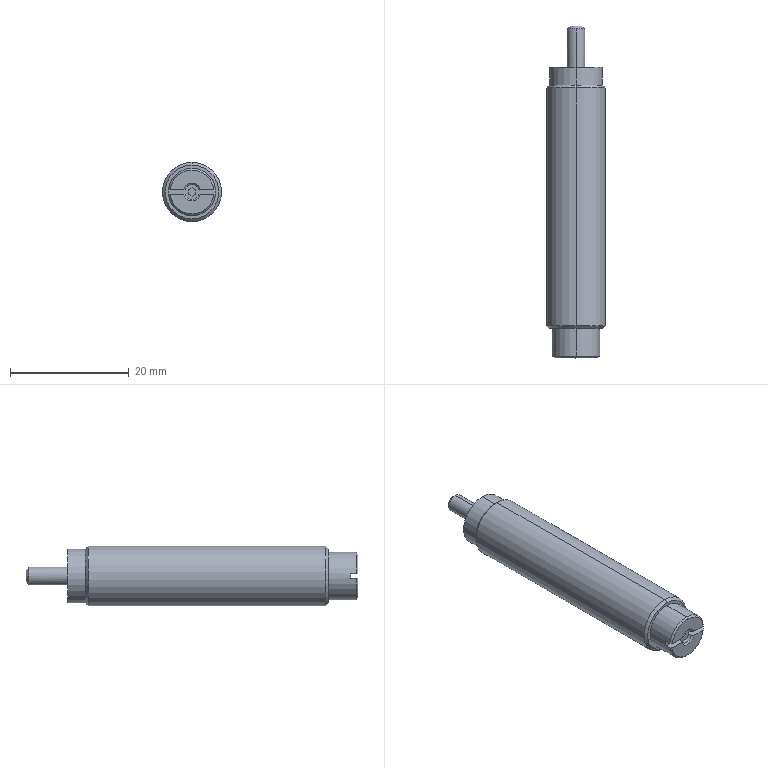Part | STEP file | 11-_ACA-1007-2-N_Body11 | 1 solid | 41 faces | box 10 x 56 x 10 mm | volume 3690 mm3 | plane 18 | cone 13 | cylinder 10 | commonest cylinder face diameters 2.459 x2 3 x2 8 x2 9 x2 10 x2
STEP:
#1=CARTESIAN_POINT('',(0.,5.46,5.));
#2=VERTEX_POINT('',#1);
#3=CARTESIAN_POINT('',(0.,5.46,-5.));
#4=VERTEX_POINT('',#3);
#5=CARTESIAN_POINT('',(0.,5.46,0.));
#6=DIRECTION('',(0.,1.,0.));
#7=DIRECTION('',(0.,0.,1.));
#8=AXIS2_PLACEMENT_3D('',#5,#6,#7);
#9=CIRCLE('',#8,5.);
#10=EDGE_CURVE('',#2,#4,#9,.T.);
#11=ORIENTED_EDGE('',*,*,#10,.T.);
#12=CARTESIAN_POINT('',(0.,45.54,-5.));
#13=VERTEX_POINT('',#12);
#14=CARTESIAN_POINT('',(0.,0.,-5.));
#15=DIRECTION('',(0.,1.,0.));
#16=VECTOR('',#15,1000.);
#17=LINE('',#14,#16);
#18=EDGE_CURVE('',#4,#13,#17,.T.);
#19=ORIENTED_EDGE('',*,*,#18,.T.);
#20=CARTESIAN_POINT('',(0.,45.54,5.));
#21=VERTEX_POINT('',#20);
#22=CARTESIAN_POINT('',(0.,45.54,0.));
#23=DIRECTION('',(0.,-1.,0.));
#24=DIRECTION('',(0.,0.,1.));
#25=AXIS2_PLACEMENT_3D('',#22,#23,#24);
#26=CIRCLE('',#25,5.);
#27=EDGE_CURVE('',#13,#21,#26,.T.);
#28=ORIENTED_EDGE('',*,*,#27,.T.);
#29=CARTESIAN_POINT('',(0.,0.,5.));
#30=DIRECTION('',(0.,1.,0.));
#31=VECTOR('',#30,1000.);
#32=LINE('',#29,#31);
#33=EDGE_CURVE('',#2,#21,#32,.T.);
#34=ORIENTED_EDGE('',*,*,#33,.F.);
#35=EDGE_LOOP('',(#11,#19,#28,#34));
#36=FACE_OUTER_BOUND('',#35,.T.);
#37=CARTESIAN_POINT('',(0.,0.,0.));
#38=DIRECTION('',(0.,1.,0.));
#39=DIRECTION('',(0.,0.,1.));
#40=AXIS2_PLACEMENT_3D('',#37,#38,#39);
#41=CYLINDRICAL_SURFACE('',#40,5.);
#42=ADVANCED_FACE('',(#36),#41,.T.);
#43=CARTESIAN_POINT('',(0.,46.,-4.54));
#44=VERTEX_POINT('',#43);
#45=CARTESIAN_POINT('',(0.,46.,4.54));
#46=VERTEX_POINT('',#45);
#47=CARTESIAN_POINT('',(0.,46.,0.));
#48=DIRECTION('',(0.,-1.,0.));
#49=DIRECTION('',(0.,0.,-1.));
#50=AXIS2_PLACEMENT_3D('',#47,#48,#49);
#51=CIRCLE('',#50,4.54);
#52=EDGE_CURVE('',#44,#46,#51,.T.);
#53=ORIENTED_EDGE('',*,*,#52,.T.);
#54=CARTESIAN_POINT('',(0.,45.54,5.));
#55=DIRECTION('',(0.,-0.7071,0.7071));
#56=VECTOR('',#55,1000.);
#57=LINE('',#54,#56);
#58=EDGE_CURVE('',#46,#21,#57,.T.);
#59=ORIENTED_EDGE('',*,*,#58,.T.);
#60=ORIENTED_EDGE('',*,*,#27,.F.);
#61=CARTESIAN_POINT('',(0.,45.54,-5.));
#62=DIRECTION('',(0.,-0.7071,-0.7071));
#63=VECTOR('',#62,1000.);
#64=LINE('',#61,#63);
#65=EDGE_CURVE('',#44,#13,#64,.T.);
#66=ORIENTED_EDGE('',*,*,#65,.F.);
#67=EDGE_LOOP('',(#53,#59,#60,#66));
#68=FACE_OUTER_BOUND('',#67,.T.);
#69=CARTESIAN_POINT('',(0.,45.54,0.));
#70=DIRECTION('',(0.,-1.,0.));
#71=DIRECTION('',(0.,0.,-1.));
#72=AXIS2_PLACEMENT_3D('',#69,#70,#71);
#73=CONICAL_SURFACE('',#72,5.,0.7854);
#74=ADVANCED_FACE('',(#68),#73,.T.);
#75=CARTESIAN_POINT('',(0.,5.,4.54));
#76=VERTEX_POINT('',#75);
#77=CARTESIAN_POINT('',(0.,5.,-4.54));
#78=VERTEX_POINT('',#77);
#79=CARTESIAN_POINT('',(0.,5.,0.));
#80=DIRECTION('',(0.,1.,0.));
#81=DIRECTION('',(0.,0.,1.));
#82=AXIS2_PLACEMENT_3D('',#79,#80,#81);
#83=CIRCLE('',#82,4.54);
#84=EDGE_CURVE('',#76,#78,#83,.T.);
#85=ORIENTED_EDGE('',*,*,#84,.T.);
#86=CARTESIAN_POINT('',(0.,5.46,-5.));
#87=DIRECTION('',(0.,0.7071,-0.7071));
#88=VECTOR('',#87,1000.);
#89=LINE('',#86,#88);
#90=EDGE_CURVE('',#78,#4,#89,.T.);
#91=ORIENTED_EDGE('',*,*,#90,.T.);
#92=ORIENTED_EDGE('',*,*,#10,.F.);
#93=CARTESIAN_POINT('',(0.,5.46,5.));
#94=DIRECTION('',(0.,0.7071,0.7071));
#95=VECTOR('',#94,1000.);
#96=LINE('',#93,#95);
#97=EDGE_CURVE('',#76,#2,#96,.T.);
#98=ORIENTED_EDGE('',*,*,#97,.F.);
#99=EDGE_LOOP('',(#85,#91,#92,#98));
#100=FACE_OUTER_BOUND('',#99,.T.);
#101=CARTESIAN_POINT('',(0.,5.46,0.));
#102=DIRECTION('',(0.,1.,0.));
#103=DIRECTION('',(0.,0.,1.));
#104=AXIS2_PLACEMENT_3D('',#101,#102,#103);
#105=CONICAL_SURFACE('',#104,5.,0.7854);
#106=ADVANCED_FACE('',(#100),#105,.T.);
#107=CARTESIAN_POINT('',(0.,46.,4.5));
#108=VERTEX_POINT('',#107);
#109=CARTESIAN_POINT('',(0.,46.,-4.5));
#110=VERTEX_POINT('',#109);
#111=CARTESIAN_POINT('',(0.,46.,0.));
#112=DIRECTION('',(0.,1.,0.));
#113=DIRECTION('',(0.,0.,1.));
#114=AXIS2_PLACEMENT_3D('',#111,#112,#113);
#115=CIRCLE('',#114,4.5);
#116=EDGE_CURVE('',#108,#110,#115,.T.);
#117=ORIENTED_EDGE('',*,*,#116,.T.);
#118=CARTESIAN_POINT('',(0.,49.,-4.5));
#119=VERTEX_POINT('',#118);
#120=CARTESIAN_POINT('',(0.,0.,-4.5));
#121=DIRECTION('',(0.,1.,0.));
#122=VECTOR('',#121,1000.);
#123=LINE('',#120,#122);
#124=EDGE_CURVE('',#110,#119,#123,.T.);
#125=ORIENTED_EDGE('',*,*,#124,.T.);
#126=CARTESIAN_POINT('',(0.,49.,4.5));
#127=VERTEX_POINT('',#126);
#128=CARTESIAN_POINT('',(0.,49.,0.));
#129=DIRECTION('',(0.,-1.,0.));
#130=DIRECTION('',(0.,0.,1.));
#131=AXIS2_PLACEMENT_3D('',#128,#129,#130);
#132=CIRCLE('',#131,4.5);
#133=EDGE_CURVE('',#119,#127,#132,.T.);
#134=ORIENTED_EDGE('',*,*,#133,.T.);
#135=CARTESIAN_POINT('',(0.,0.,4.5));
#136=DIRECTION('',(0.,1.,0.));
#137=VECTOR('',#136,1000.);
#138=LINE('',#135,#137);
#139=EDGE_CURVE('',#108,#127,#138,.T.);
#140=ORIENTED_EDGE('',*,*,#139,.F.);
#141=EDGE_LOOP('',(#117,#125,#134,#140));
#142=FACE_OUTER_BOUND('',#141,.T.);
#143=CARTESIAN_POINT('',(0.,0.,0.));
#144=DIRECTION('',(0.,1.,0.));
#145=DIRECTION('',(0.,0.,1.));
#146=AXIS2_PLACEMENT_3D('',#143,#144,#145);
#147=CYLINDRICAL_SURFACE('',#146,4.5);
#148=ADVANCED_FACE('',(#142),#147,.T.);
#149=CARTESIAN_POINT('',(3.98,0.3,-0.4));
#150=VERTEX_POINT('',#149);
#151=CARTESIAN_POINT('',(0.,0.3,-4.));
#152=VERTEX_POINT('',#151);
#153=CARTESIAN_POINT('',(0.,0.3,0.));
#154=DIRECTION('',(0.,1.,0.));
#155=DIRECTION('',(0.,0.,1.));
#156=AXIS2_PLACEMENT_3D('',#153,#154,#155);
#157=CIRCLE('',#156,4.);
#158=EDGE_CURVE('',#150,#152,#157,.T.);
#159=ORIENTED_EDGE('',*,*,#158,.T.);
#160=CARTESIAN_POINT('',(0.,5.,-4.));
#161=VERTEX_POINT('',#160);
#162=CARTESIAN_POINT('',(0.,0.,-4.));
#163=DIRECTION('',(0.,1.,0.));
#164=VECTOR('',#163,1000.);
#165=LINE('',#162,#164);
#166=EDGE_CURVE('',#152,#161,#165,.T.);
#167=ORIENTED_EDGE('',*,*,#166,.T.);
#168=CARTESIAN_POINT('',(0.,5.,4.));
#169=VERTEX_POINT('',#168);
#170=CARTESIAN_POINT('',(0.,5.,0.));
#171=DIRECTION('',(0.,-1.,0.));
#172=DIRECTION('',(0.,0.,1.));
#173=AXIS2_PLACEMENT_3D('',#170,#171,#172);
#174=CIRCLE('',#173,4.);
#175=EDGE_CURVE('',#161,#169,#174,.T.);
#176=ORIENTED_EDGE('',*,*,#175,.T.);
#177=CARTESIAN_POINT('',(0.,0.3,4.));
#178=VERTEX_POINT('',#177);
#179=CARTESIAN_POINT('',(0.,0.,4.));
#180=DIRECTION('',(0.,1.,0.));
#181=VECTOR('',#180,1000.);
#182=LINE('',#179,#181);
#183=EDGE_CURVE('',#178,#169,#182,.T.);
#184=ORIENTED_EDGE('',*,*,#183,.F.);
#185=CARTESIAN_POINT('',(3.98,0.3,0.4));
#186=VERTEX_POINT('',#185);
#187=CARTESIAN_POINT('',(0.,0.3,0.));
#188=DIRECTION('',(0.,1.,0.));
#189=DIRECTION('',(0.,0.,1.));
#190=AXIS2_PLACEMENT_3D('',#187,#188,#189);
#191=CIRCLE('',#190,4.);
#192=EDGE_CURVE('',#178,#186,#191,.T.);
#193=ORIENTED_EDGE('',*,*,#192,.T.);
#194=CARTESIAN_POINT('',(3.98,1.2,0.4));
#195=VERTEX_POINT('',#194);
#196=CARTESIAN_POINT('',(3.98,0.,0.4));
#197=DIRECTION('',(0.,1.,0.));
#198=VECTOR('',#197,1000.);
#199=LINE('',#196,#198);
#200=EDGE_CURVE('',#186,#195,#199,.T.);
#201=ORIENTED_EDGE('',*,*,#200,.T.);
#202=CARTESIAN_POINT('',(3.98,1.2,-0.4));
#203=VERTEX_POINT('',#202);
#204=CARTESIAN_POINT('',(0.,1.2,0.));
#205=DIRECTION('',(0.,-1.,0.));
#206=DIRECTION('',(0.,0.,1.));
#207=AXIS2_PLACEMENT_3D('',#204,#205,#206);
#208=CIRCLE('',#207,4.);
#209=EDGE_CURVE('',#203,#195,#208,.T.);
#210=ORIENTED_EDGE('',*,*,#209,.F.);
#211=CARTESIAN_POINT('',(3.98,0.,-0.4));
#212=DIRECTION('',(0.,1.,0.));
#213=VECTOR('',#212,1000.);
#214=LINE('',#211,#213);
#215=EDGE_CURVE('',#150,#203,#214,.T.);
#216=ORIENTED_EDGE('',*,*,#215,.F.);
#217=EDGE_LOOP('',(#159,#167,#176,#184,#193,#201,#210,#216));
#218=FACE_OUTER_BOUND('',#217,.T.);
#219=CARTESIAN_POINT('',(0.,0.,0.));
#220=DIRECTION('',(0.,1.,0.));
#221=DIRECTION('',(0.,0.,1.));
#222=AXIS2_PLACEMENT_3D('',#219,#220,#221);
#223=CYLINDRICAL_SURFACE('',#222,4.);
#224=ADVANCED_FACE('',(#218),#223,.T.);
#225=CARTESIAN_POINT('',(-3.678,0.,0.4));
#226=VERTEX_POINT('',#225);
#227=CARTESIAN_POINT('',(0.,0.,3.7));
#228=VERTEX_POINT('',#227);
#229=CARTESIAN_POINT('',(0.,0.,0.));
#230=DIRECTION('',(0.,1.,0.));
#231=DIRECTION('',(0.,0.,1.));
#232=AXIS2_PLACEMENT_3D('',#229,#230,#231);
#233=CIRCLE('',#232,3.7);
#234=EDGE_CURVE('',#226,#228,#233,.T.);
#235=ORIENTED_EDGE('',*,*,#234,.T.);
#236=CARTESIAN_POINT('',(0.,0.3,4.));
#237=DIRECTION('',(0.,0.7071,0.7071));
#238=VECTOR('',#237,1000.);
#239=LINE('',#236,#238);
#240=EDGE_CURVE('',#228,#178,#239,.T.);
#241=ORIENTED_EDGE('',*,*,#240,.T.);
#242=CARTESIAN_POINT('',(-3.98,0.3,0.4));
#243=VERTEX_POINT('',#242);
#244=CARTESIAN_POINT('',(0.,0.3,0.));
#245=DIRECTION('',(0.,1.,0.));
#246=DIRECTION('',(0.,0.,1.));
#247=AXIS2_PLACEMENT_3D('',#244,#245,#246);
#248=CIRCLE('',#247,4.);
#249=EDGE_CURVE('',#243,#178,#248,.T.);
#250=ORIENTED_EDGE('',*,*,#249,.F.);
#251=CARTESIAN_POINT('',(-3.98,0.3,0.4));
#252=CARTESIAN_POINT('',(-3.879,0.2,0.4));
#253=CARTESIAN_POINT('',(-3.779,0.09998,0.4));
#254=CARTESIAN_POINT('',(-3.678,0.,0.4));
#255=B_SPLINE_CURVE_WITH_KNOTS('',3,(#251,#252,#253,#254),.UNSPECIFIED.,.F.,.F.,(4,4),(0.,0.0004254),.UNSPECIFIED.);
#256=EDGE_CURVE('',#243,#226,#255,.T.);
#257=ORIENTED_EDGE('',*,*,#256,.T.);
#258=EDGE_LOOP('',(#235,#241,#250,#257));
#259=FACE_OUTER_BOUND('',#258,.T.);
#260=CARTESIAN_POINT('',(0.,0.3,0.));
#261=DIRECTION('',(0.,1.,0.));
#262=DIRECTION('',(0.,0.,1.));
#263=AXIS2_PLACEMENT_3D('',#260,#261,#262);
#264=CONICAL_SURFACE('',#263,4.,0.7854);
#265=ADVANCED_FACE('',(#259),#264,.T.);
#266=CARTESIAN_POINT('',(0.,49.,1.5));
#267=VERTEX_POINT('',#266);
#268=CARTESIAN_POINT('',(0.,49.,-1.5));
#269=VERTEX_POINT('',#268);
#270=CARTESIAN_POINT('',(0.,49.,0.));
#271=DIRECTION('',(0.,1.,0.));
#272=DIRECTION('',(0.,0.,1.));
#273=AXIS2_PLACEMENT_3D('',#270,#271,#272);
#274=CIRCLE('',#273,1.5);
#275=EDGE_CURVE('',#267,#269,#274,.T.);
#276=ORIENTED_EDGE('',*,*,#275,.T.);
#277=CARTESIAN_POINT('',(0.,55.5,-1.5));
#278=VERTEX_POINT('',#277);
#279=CARTESIAN_POINT('',(0.,0.,-1.5));
#280=DIRECTION('',(0.,1.,0.));
#281=VECTOR('',#280,1000.);
#282=LINE('',#279,#281);
#283=EDGE_CURVE('',#269,#278,#282,.T.);
#284=ORIENTED_EDGE('',*,*,#283,.T.);
#285=CARTESIAN_POINT('',(1.5,55.5,0.));
#286=VERTEX_POINT('',#285);
#287=CARTESIAN_POINT('',(0.,55.5,0.));
#288=DIRECTION('',(0.,-1.,0.));
#289=DIRECTION('',(0.,0.,1.));
#290=AXIS2_PLACEMENT_3D('',#287,#288,#289);
#291=CIRCLE('',#290,1.5);
#292=EDGE_CURVE('',#278,#286,#291,.T.);
#293=ORIENTED_EDGE('',*,*,#292,.T.);
#294=CARTESIAN_POINT('',(0.,55.5,1.5));
#295=VERTEX_POINT('',#294);
#296=CARTESIAN_POINT('',(0.,55.5,0.));
#297=DIRECTION('',(0.,-1.,0.));
#298=DIRECTION('',(0.,0.,1.));
#299=AXIS2_PLACEMENT_3D('',#296,#297,#298);
#300=CIRCLE('',#299,1.5);
#301=EDGE_CURVE('',#286,#295,#300,.T.);
#302=ORIENTED_EDGE('',*,*,#301,.T.);
#303=CARTESIAN_POINT('',(0.,0.,1.5));
#304=DIRECTION('',(0.,1.,0.));
#305=VECTOR('',#304,1000.);
#306=LINE('',#303,#305);
#307=EDGE_CURVE('',#267,#295,#306,.T.);
#308=ORIENTED_EDGE('',*,*,#307,.F.);
#309=EDGE_LOOP('',(#276,#284,#293,#302,#308));
#310=FACE_OUTER_BOUND('',#309,.T.);
#311=CARTESIAN_POINT('',(0.,0.,0.));
#312=DIRECTION('',(0.,1.,0.));
#313=DIRECTION('',(0.,0.,1.));
#314=AXIS2_PLACEMENT_3D('',#311,#312,#313);
#315=CYLINDRICAL_SURFACE('',#314,1.5);
#316=ADVANCED_FACE('',(#310),#315,.T.);
#317=CARTESIAN_POINT('',(1.,56.,0.));
#318=VERTEX_POINT('',#317);
#319=CARTESIAN_POINT('',(-1.,56.,0.));
#320=VERTEX_POINT('',#319);
#321=CARTESIAN_POINT('',(0.,56.,0.));
#322=DIRECTION('',(0.,-1.,0.));
#323=DIRECTION('',(1.,0.,0.));
#324=AXIS2_PLACEMENT_3D('',#321,#322,#323);
#325=CIRCLE('',#324,1.);
#326=EDGE_CURVE('',#318,#320,#325,.T.);
#327=ORIENTED_EDGE('',*,*,#326,.T.);
#328=CARTESIAN_POINT('',(-1.5,55.5,0.));
#329=VERTEX_POINT('',#328);
#330=CARTESIAN_POINT('',(-1.5,55.5,0.));
#331=DIRECTION('',(-0.7071,-0.7071,0.));
#332=VECTOR('',#331,1000.);
#333=LINE('',#330,#332);
#334=EDGE_CURVE('',#320,#329,#333,.T.);
#335=ORIENTED_EDGE('',*,*,#334,.T.);
#336=CARTESIAN_POINT('',(0.,55.5,0.));
#337=DIRECTION('',(0.,-1.,0.));
#338=DIRECTION('',(0.,0.,1.));
#339=AXIS2_PLACEMENT_3D('',#336,#337,#338);
#340=CIRCLE('',#339,1.5);
#341=EDGE_CURVE('',#295,#329,#340,.T.);
#342=ORIENTED_EDGE('',*,*,#341,.F.);
#343=ORIENTED_EDGE('',*,*,#301,.F.);
#344=CARTESIAN_POINT('',(1.5,55.5,0.));
#345=DIRECTION('',(0.7071,-0.7071,0.));
#346=VECTOR('',#345,1000.);
#347=LINE('',#344,#346);
#348=EDGE_CURVE('',#318,#286,#347,.T.);
#349=ORIENTED_EDGE('',*,*,#348,.F.);
#350=EDGE_LOOP('',(#327,#335,#342,#343,#349));
#351=FACE_OUTER_BOUND('',#350,.T.);
#352=CARTESIAN_POINT('',(0.,55.5,0.));
#353=DIRECTION('',(0.,-1.,0.));
#354=DIRECTION('',(1.,0.,0.));
#355=AXIS2_PLACEMENT_3D('',#352,#353,#354);
#356=CONICAL_SURFACE('',#355,1.5,0.7854);
#357=ADVANCED_FACE('',(#351),#356,.T.);
#358=ORIENTED_EDGE('',*,*,#18,.F.);
#359=CARTESIAN_POINT('',(0.,5.46,0.));
#360=DIRECTION('',(0.,1.,0.));
#361=DIRECTION('',(0.,0.,1.));
#362=AXIS2_PLACEMENT_3D('',#359,#360,#361);
#363=CIRCLE('',#362,5.);
#364=EDGE_CURVE('',#4,#2,#363,.T.);
#365=ORIENTED_EDGE('',*,*,#364,.T.);
#366=ORIENTED_EDGE('',*,*,#33,.T.);
#367=CARTESIAN_POINT('',(0.,45.54,0.));
#368=DIRECTION('',(0.,-1.,0.));
#369=DIRECTION('',(0.,0.,1.));
#370=AXIS2_PLACEMENT_3D('',#367,#368,#369);
#371=CIRCLE('',#370,5.);
#372=EDGE_CURVE('',#21,#13,#371,.T.);
#373=ORIENTED_EDGE('',*,*,#372,.T.);
#374=EDGE_LOOP('',(#358,#365,#366,#373));
#375=FACE_OUTER_BOUND('',#374,.T.);
#376=CARTESIAN_POINT('',(0.,0.,0.));
#377=DIRECTION('',(0.,1.,0.));
#378=DIRECTION('',(0.,0.,1.));
#379=AXIS2_PLACEMENT_3D('',#376,#377,#378);
#380=CYLINDRICAL_SURFACE('',#379,5.);
#381=ADVANCED_FACE('',(#375),#380,.T.);
#382=ORIENTED_EDGE('',*,*,#58,.F.);
#383=CARTESIAN_POINT('',(0.,46.,0.));
#384=DIRECTION('',(0.,-1.,0.));
#385=DIRECTION('',(0.,0.,-1.));
#386=AXIS2_PLACEMENT_3D('',#383,#384,#385);
#387=CIRCLE('',#386,4.54);
#388=EDGE_CURVE('',#46,#44,#387,.T.);
#389=ORIENTED_EDGE('',*,*,#388,.T.);
#390=ORIENTED_EDGE('',*,*,#65,.T.);
#391=ORIENTED_EDGE('',*,*,#372,.F.);
#392=EDGE_LOOP('',(#382,#389,#390,#391));
#393=FACE_OUTER_BOUND('',#392,.T.);
#394=CARTESIAN_POINT('',(0.,45.54,0.));
#395=DIRECTION('',(0.,-1.,0.));
#396=DIRECTION('',(0.,0.,-1.));
#397=AXIS2_PLACEMENT_3D('',#394,#395,#396);
#398=CONICAL_SURFACE('',#397,5.,0.7854);
#399=ADVANCED_FACE('',(#393),#398,.T.);
#400=ORIENTED_EDGE('',*,*,#90,.F.);
#401=CARTESIAN_POINT('',(0.,5.,0.));
#402=DIRECTION('',(0.,1.,0.));
#403=DIRECTION('',(0.,0.,1.));
#404=AXIS2_PLACEMENT_3D('',#401,#402,#403);
#405=CIRCLE('',#404,4.54);
#406=EDGE_CURVE('',#78,#76,#405,.T.);
#407=ORIENTED_EDGE('',*,*,#406,.T.);
#408=ORIENTED_EDGE('',*,*,#97,.T.);
#409=ORIENTED_EDGE('',*,*,#364,.F.);
#410=EDGE_LOOP('',(#400,#407,#408,#409));
#411=FACE_OUTER_BOUND('',#410,.T.);
#412=CARTESIAN_POINT('',(0.,5.46,0.));
#413=DIRECTION('',(0.,1.,0.));
#414=DIRECTION('',(0.,0.,1.));
#415=AXIS2_PLACEMENT_3D('',#412,#413,#414);
#416=CONICAL_SURFACE('',#415,5.,0.7854);
#417=ADVANCED_FACE('',(#411),#416,.T.);
#418=ORIENTED_EDGE('',*,*,#116,.F.);
#419=CARTESIAN_POINT('',(0.,46.,0.));
#420=DIRECTION('',(0.,1.,0.));
#421=DIRECTION('',(0.,0.,1.));
#422=AXIS2_PLACEMENT_3D('',#419,#420,#421);
#423=CIRCLE('',#422,4.5);
#424=EDGE_CURVE('',#110,#108,#423,.T.);
#425=ORIENTED_EDGE('',*,*,#424,.F.);
#426=EDGE_LOOP('',(#418,#425));
#427=FACE_BOUND('',#426,.T.);
#428=ORIENTED_EDGE('',*,*,#52,.F.);
#429=ORIENTED_EDGE('',*,*,#388,.F.);
#430=EDGE_LOOP('',(#428,#429));
#431=FACE_OUTER_BOUND('',#430,.T.);
#432=CARTESIAN_POINT('',(4.5,46.,0.));
#433=DIRECTION('',(0.,-1.,0.));
#434=DIRECTION('',(0.,0.,-1.));
#435=AXIS2_PLACEMENT_3D('',#432,#433,#434);
#436=PLANE('',#435);
#437=ADVANCED_FACE('',(#427,#431),#436,.F.);
#438=ORIENTED_EDGE('',*,*,#84,.F.);
#439=ORIENTED_EDGE('',*,*,#406,.F.);
#440=EDGE_LOOP('',(#438,#439));
#441=FACE_OUTER_BOUND('',#440,.T.);
#442=CARTESIAN_POINT('',(0.,5.,0.));
#443=DIRECTION('',(0.,-1.,0.));
#444=DIRECTION('',(0.,0.,1.));
#445=AXIS2_PLACEMENT_3D('',#442,#443,#444);
#446=CIRCLE('',#445,4.);
#447=EDGE_CURVE('',#169,#161,#446,.T.);
#448=ORIENTED_EDGE('',*,*,#447,.F.);
#449=ORIENTED_EDGE('',*,*,#175,.F.);
#450=EDGE_LOOP('',(#448,#449));
#451=FACE_BOUND('',#450,.T.);
#452=CARTESIAN_POINT('',(4.54,5.,0.));
#453=DIRECTION('',(0.,1.,0.));
#454=DIRECTION('',(0.,0.,1.));
#455=AXIS2_PLACEMENT_3D('',#452,#453,#454);
#456=PLANE('',#455);
#457=ADVANCED_FACE('',(#441,#451),#456,.F.);
#458=ORIENTED_EDGE('',*,*,#124,.F.);
#459=ORIENTED_EDGE('',*,*,#424,.T.);
#460=ORIENTED_EDGE('',*,*,#139,.T.);
#461=CARTESIAN_POINT('',(0.,49.,0.));
#462=DIRECTION('',(0.,-1.,0.));
#463=DIRECTION('',(0.,0.,1.));
#464=AXIS2_PLACEMENT_3D('',#461,#462,#463);
#465=CIRCLE('',#464,4.5);
#466=EDGE_CURVE('',#127,#119,#465,.T.);
#467=ORIENTED_EDGE('',*,*,#466,.T.);
#468=EDGE_LOOP('',(#458,#459,#460,#467));
#469=FACE_OUTER_BOUND('',#468,.T.);
#470=CARTESIAN_POINT('',(0.,0.,0.));
#471=DIRECTION('',(0.,1.,0.));
#472=DIRECTION('',(0.,0.,1.));
#473=AXIS2_PLACEMENT_3D('',#470,#471,#472);
#474=CYLINDRICAL_SURFACE('',#473,4.5);
#475=ADVANCED_FACE('',(#469),#474,.T.);
#476=ORIENTED_EDGE('',*,*,#166,.F.);
#477=CARTESIAN_POINT('',(-3.98,0.3,-0.4));
#478=VERTEX_POINT('',#477);
#479=CARTESIAN_POINT('',(0.,0.3,0.));
#480=DIRECTION('',(0.,1.,0.));
#481=DIRECTION('',(0.,0.,1.));
#482=AXIS2_PLACEMENT_3D('',#479,#480,#481);
#483=CIRCLE('',#482,4.);
#484=EDGE_CURVE('',#152,#478,#483,.T.);
#485=ORIENTED_EDGE('',*,*,#484,.T.);
#486=CARTESIAN_POINT('',(-3.98,1.2,-0.4));
#487=VERTEX_POINT('',#486);
#488=CARTESIAN_POINT('',(-3.98,0.,-0.4));
#489=DIRECTION('',(0.,-1.,0.));
#490=VECTOR('',#489,1000.);
#491=LINE('',#488,#490);
#492=EDGE_CURVE('',#487,#478,#491,.T.);
#493=ORIENTED_EDGE('',*,*,#492,.F.);
#494=CARTESIAN_POINT('',(-3.98,1.2,0.4));
#495=VERTEX_POINT('',#494);
#496=CARTESIAN_POINT('',(0.,1.2,0.));
#497=DIRECTION('',(0.,-1.,0.));
#498=DIRECTION('',(0.,0.,1.));
#499=AXIS2_PLACEMENT_3D('',#496,#497,#498);
#500=CIRCLE('',#499,4.);
#501=EDGE_CURVE('',#495,#487,#500,.T.);
#502=ORIENTED_EDGE('',*,*,#501,.F.);
#503=CARTESIAN_POINT('',(-3.98,0.,0.4));
#504=DIRECTION('',(0.,-1.,0.));
#505=VECTOR('',#504,1000.);
#506=LINE('',#503,#505);
#507=EDGE_CURVE('',#495,#243,#506,.T.);
#508=ORIENTED_EDGE('',*,*,#507,.T.);
#509=ORIENTED_EDGE('',*,*,#249,.T.);
#510=ORIENTED_EDGE('',*,*,#183,.T.);
#511=ORIENTED_EDGE('',*,*,#447,.T.);
#512=EDGE_LOOP('',(#476,#485,#493,#502,#508,#509,#510,#511));
#513=FACE_OUTER_BOUND('',#512,.T.);
#514=CARTESIAN_POINT('',(0.,0.,0.));
#515=DIRECTION('',(0.,1.,0.));
#516=DIRECTION('',(0.,0.,1.));
#517=AXIS2_PLACEMENT_3D('',#514,#515,#516);
#518=CYLINDRICAL_SURFACE('',#517,4.);
#519=ADVANCED_FACE('',(#513),#518,.T.);
#520=ORIENTED_EDGE('',*,*,#275,.F.);
#521=CARTESIAN_POINT('',(0.,49.,0.));
#522=DIRECTION('',(0.,1.,0.));
#523=DIRECTION('',(0.,0.,1.));
#524=AXIS2_PLACEMENT_3D('',#521,#522,#523);
#525=CIRCLE('',#524,1.5);
#526=EDGE_CURVE('',#269,#267,#525,.T.);
#527=ORIENTED_EDGE('',*,*,#526,.F.);
#528=EDGE_LOOP('',(#520,#527));
#529=FACE_BOUND('',#528,.T.);
#530=ORIENTED_EDGE('',*,*,#466,.F.);
#531=ORIENTED_EDGE('',*,*,#133,.F.);
#532=EDGE_LOOP('',(#530,#531));
#533=FACE_OUTER_BOUND('',#532,.T.);
#534=CARTESIAN_POINT('',(1.5,49.,0.));
#535=DIRECTION('',(0.,-1.,0.));
#536=DIRECTION('',(0.,0.,-1.));
#537=AXIS2_PLACEMENT_3D('',#534,#535,#536);
#538=PLANE('',#537);
#539=ADVANCED_FACE('',(#529,#533),#538,.F.);
#540=ORIENTED_EDGE('',*,*,#240,.F.);
#541=CARTESIAN_POINT('',(3.678,0.,0.4));
#542=VERTEX_POINT('',#541);
#543=CARTESIAN_POINT('',(0.,0.,0.));
#544=DIRECTION('',(0.,1.,0.));
#545=DIRECTION('',(0.,0.,1.));
#546=AXIS2_PLACEMENT_3D('',#543,#544,#545);
#547=CIRCLE('',#546,3.7);
#548=EDGE_CURVE('',#228,#542,#547,.T.);
#549=ORIENTED_EDGE('',*,*,#548,.T.);
#550=CARTESIAN_POINT('',(3.678,0.,0.4));
#551=CARTESIAN_POINT('',(3.779,0.09998,0.4));
#552=CARTESIAN_POINT('',(3.879,0.2,0.4));
#553=CARTESIAN_POINT('',(3.98,0.3,0.4));
#554=B_SPLINE_CURVE_WITH_KNOTS('',3,(#550,#551,#552,#553),.UNSPECIFIED.,.F.,.F.,(4,4),(0.,0.0004254),.UNSPECIFIED.);
#555=EDGE_CURVE('',#542,#186,#554,.T.);
#556=ORIENTED_EDGE('',*,*,#555,.T.);
#557=ORIENTED_EDGE('',*,*,#192,.F.);
#558=EDGE_LOOP('',(#540,#549,#556,#557));
#559=FACE_OUTER_BOUND('',#558,.T.);
#560=CARTESIAN_POINT('',(0.,0.3,0.));
#561=DIRECTION('',(0.,1.,0.));
#562=DIRECTION('',(0.,0.,1.));
#563=AXIS2_PLACEMENT_3D('',#560,#561,#562);
#564=CONICAL_SURFACE('',#563,4.,0.7854);
#565=ADVANCED_FACE('',(#559),#564,.T.);
#566=CARTESIAN_POINT('',(3.678,0.,-0.4));
#567=VERTEX_POINT('',#566);
#568=CARTESIAN_POINT('',(3.678,0.,-0.4));
#569=CARTESIAN_POINT('',(3.779,0.09998,-0.4));
#570=CARTESIAN_POINT('',(3.879,0.2,-0.4));
#571=CARTESIAN_POINT('',(3.98,0.3,-0.4));
#572=B_SPLINE_CURVE_WITH_KNOTS('',3,(#568,#569,#570,#571),.UNSPECIFIED.,.F.,.F.,(4,4),(0.,0.0004254),.UNSPECIFIED.);
#573=EDGE_CURVE('',#567,#150,#572,.T.);
#574=ORIENTED_EDGE('',*,*,#573,.F.);
#575=CARTESIAN_POINT('',(-3.678,0.,-0.4));
#576=VERTEX_POINT('',#575);
#577=CARTESIAN_POINT('',(0.,0.,0.));
#578=DIRECTION('',(0.,1.,0.));
#579=DIRECTION('',(0.,0.,1.));
#580=AXIS2_PLACEMENT_3D('',#577,#578,#579);
#581=CIRCLE('',#580,3.7);
#582=EDGE_CURVE('',#567,#576,#581,.T.);
#583=ORIENTED_EDGE('',*,*,#582,.T.);
#584=CARTESIAN_POINT('',(-3.98,0.3,-0.4));
#585=CARTESIAN_POINT('',(-3.879,0.2,-0.4));
#586=CARTESIAN_POINT('',(-3.779,0.09998,-0.4));
#587=CARTESIAN_POINT('',(-3.678,0.,-0.4));
#588=B_SPLINE_CURVE_WITH_KNOTS('',3,(#584,#585,#586,#587),.UNSPECIFIED.,.F.,.F.,(4,4),(0.,0.0004254),.UNSPECIFIED.);
#589=EDGE_CURVE('',#478,#576,#588,.T.);
#590=ORIENTED_EDGE('',*,*,#589,.F.);
#591=ORIENTED_EDGE('',*,*,#484,.F.);
#592=ORIENTED_EDGE('',*,*,#158,.F.);
#593=EDGE_LOOP('',(#574,#583,#590,#591,#592));
#594=FACE_OUTER_BOUND('',#593,.T.);
#595=CARTESIAN_POINT('',(0.,0.3,0.));
#596=DIRECTION('',(0.,1.,0.));
#597=DIRECTION('',(0.,0.,1.));
#598=AXIS2_PLACEMENT_3D('',#595,#596,#597);
#599=CONICAL_SURFACE('',#598,4.,0.7854);
#600=ADVANCED_FACE('',(#594),#599,.T.);
#601=ORIENTED_EDGE('',*,*,#283,.F.);
#602=ORIENTED_EDGE('',*,*,#526,.T.);
#603=ORIENTED_EDGE('',*,*,#307,.T.);
#604=ORIENTED_EDGE('',*,*,#341,.T.);
#605=CARTESIAN_POINT('',(0.,55.5,0.));
#606=DIRECTION('',(0.,-1.,0.));
#607=DIRECTION('',(0.,0.,1.));
#608=AXIS2_PLACEMENT_3D('',#605,#606,#607);
#609=CIRCLE('',#608,1.5);
#610=EDGE_CURVE('',#329,#278,#609,.T.);
#611=ORIENTED_EDGE('',*,*,#610,.T.);
#612=EDGE_LOOP('',(#601,#602,#603,#604,#611));
#613=FACE_OUTER_BOUND('',#612,.T.);
#614=CARTESIAN_POINT('',(0.,0.,0.));
#615=DIRECTION('',(0.,1.,0.));
#616=DIRECTION('',(0.,0.,1.));
#617=AXIS2_PLACEMENT_3D('',#614,#615,#616);
#618=CYLINDRICAL_SURFACE('',#617,1.5);
#619=ADVANCED_FACE('',(#613),#618,.T.);
#620=CARTESIAN_POINT('',(-1.446,0.,0.4));
#621=VERTEX_POINT('',#620);
#622=CARTESIAN_POINT('',(3.7,0.,0.4));
#623=DIRECTION('',(-1.,0.,0.));
#624=VECTOR('',#623,1000.);
#625=LINE('',#622,#624);
#626=EDGE_CURVE('',#621,#226,#625,.T.);
#627=ORIENTED_EDGE('',*,*,#626,.F.);
#628=CARTESIAN_POINT('',(1.446,0.,0.4));
#629=VERTEX_POINT('',#628);
#630=CARTESIAN_POINT('',(0.,0.,0.));
#631=DIRECTION('',(0.,-1.,0.));
#632=DIRECTION('',(1.,0.,0.));
#633=AXIS2_PLACEMENT_3D('',#630,#631,#632);
#634=CIRCLE('',#633,1.5);
#635=EDGE_CURVE('',#629,#621,#634,.T.);
#636=ORIENTED_EDGE('',*,*,#635,.F.);
#637=CARTESIAN_POINT('',(3.7,0.,0.4));
#638=DIRECTION('',(-1.,0.,0.));
#639=VECTOR('',#638,1000.);
#640=LINE('',#637,#639);
#641=EDGE_CURVE('',#542,#629,#640,.T.);
#642=ORIENTED_EDGE('',*,*,#641,.F.);
#643=ORIENTED_EDGE('',*,*,#548,.F.);
#644=ORIENTED_EDGE('',*,*,#234,.F.);
#645=EDGE_LOOP('',(#627,#636,#642,#643,#644));
#646=FACE_OUTER_BOUND('',#645,.T.);
#647=CARTESIAN_POINT('',(3.7,0.,0.));
#648=DIRECTION('',(0.,1.,0.));
#649=DIRECTION('',(0.,0.,1.));
#650=AXIS2_PLACEMENT_3D('',#647,#648,#649);
#651=PLANE('',#650);
#652=ADVANCED_FACE('',(#646),#651,.F.);
#653=ORIENTED_EDGE('',*,*,#582,.F.);
#654=CARTESIAN_POINT('',(1.446,0.,-0.4));
#655=VERTEX_POINT('',#654);
#656=CARTESIAN_POINT('',(3.7,0.,-0.4));
#657=DIRECTION('',(1.,0.,0.));
#658=VECTOR('',#657,1000.);
#659=LINE('',#656,#658);
#660=EDGE_CURVE('',#655,#567,#659,.T.);
#661=ORIENTED_EDGE('',*,*,#660,.F.);
#662=CARTESIAN_POINT('',(-1.446,0.,-0.4));
#663=VERTEX_POINT('',#662);
#664=CARTESIAN_POINT('',(0.,0.,0.));
#665=DIRECTION('',(0.,-1.,0.));
#666=DIRECTION('',(1.,0.,0.));
#667=AXIS2_PLACEMENT_3D('',#664,#665,#666);
#668=CIRCLE('',#667,1.5);
#669=EDGE_CURVE('',#663,#655,#668,.T.);
#670=ORIENTED_EDGE('',*,*,#669,.F.);
#671=CARTESIAN_POINT('',(3.7,0.,-0.4));
#672=DIRECTION('',(1.,0.,0.));
#673=VECTOR('',#672,1000.);
#674=LINE('',#671,#673);
#675=EDGE_CURVE('',#576,#663,#674,.T.);
#676=ORIENTED_EDGE('',*,*,#675,.F.);
#677=EDGE_LOOP('',(#653,#661,#670,#676));
#678=FACE_OUTER_BOUND('',#677,.T.);
#679=CARTESIAN_POINT('',(3.7,0.,0.));
#680=DIRECTION('',(0.,1.,0.));
#681=DIRECTION('',(0.,0.,1.));
#682=AXIS2_PLACEMENT_3D('',#679,#680,#681);
#683=PLANE('',#682);
#684=ADVANCED_FACE('',(#678),#683,.F.);
#685=ORIENTED_EDGE('',*,*,#334,.F.);
#686=CARTESIAN_POINT('',(0.,56.,0.));
#687=DIRECTION('',(0.,-1.,0.));
#688=DIRECTION('',(1.,0.,0.));
#689=AXIS2_PLACEMENT_3D('',#686,#687,#688);
#690=CIRCLE('',#689,1.);
#691=EDGE_CURVE('',#320,#318,#690,.T.);
#692=ORIENTED_EDGE('',*,*,#691,.T.);
#693=ORIENTED_EDGE('',*,*,#348,.T.);
#694=ORIENTED_EDGE('',*,*,#292,.F.);
#695=ORIENTED_EDGE('',*,*,#610,.F.);
#696=EDGE_LOOP('',(#685,#692,#693,#694,#695));
#697=FACE_OUTER_BOUND('',#696,.T.);
#698=CARTESIAN_POINT('',(0.,55.5,0.));
#699=DIRECTION('',(0.,-1.,0.));
#700=DIRECTION('',(1.,0.,0.));
#701=AXIS2_PLACEMENT_3D('',#698,#699,#700);
#702=CONICAL_SURFACE('',#701,1.5,0.7854);
#703=ADVANCED_FACE('',(#697),#702,.T.);
#704=CARTESIAN_POINT('',(-1.446,1.2,0.4));
#705=VERTEX_POINT('',#704);
#706=CARTESIAN_POINT('',(-1.163,0.9295,0.4));
#707=VERTEX_POINT('',#706);
#708=CARTESIAN_POINT('',(-1.446,1.2,0.4));
#709=CARTESIAN_POINT('',(-1.352,1.109,0.4));
#710=CARTESIAN_POINT('',(-1.257,1.019,0.4));
#711=CARTESIAN_POINT('',(-1.163,0.9295,0.4));
#712=B_SPLINE_CURVE_WITH_KNOTS('',3,(#708,#709,#710,#711),.UNSPECIFIED.,.F.,.F.,(4,4),(0.,0.0003915),.UNSPECIFIED.);
#713=EDGE_CURVE('',#705,#707,#712,.T.);
#714=ORIENTED_EDGE('',*,*,#713,.T.);
#715=CARTESIAN_POINT('',(-1.163,0.2705,0.4));
#716=VERTEX_POINT('',#715);
#717=CARTESIAN_POINT('',(-1.163,0.,0.4));
#718=DIRECTION('',(0.,-1.,0.));
#719=VECTOR('',#718,1000.);
#720=LINE('',#717,#719);
#721=EDGE_CURVE('',#707,#716,#720,.T.);
#722=ORIENTED_EDGE('',*,*,#721,.T.);
#723=CARTESIAN_POINT('',(-1.446,0.,0.4));
#724=CARTESIAN_POINT('',(-1.352,0.09057,0.4));
#725=CARTESIAN_POINT('',(-1.257,0.1808,0.4));
#726=CARTESIAN_POINT('',(-1.163,0.2705,0.4));
#727=B_SPLINE_CURVE_WITH_KNOTS('',3,(#723,#724,#725,#726),.UNSPECIFIED.,.F.,.F.,(4,4),(0.,0.0003915),.UNSPECIFIED.);
#728=EDGE_CURVE('',#621,#716,#727,.T.);
#729=ORIENTED_EDGE('',*,*,#728,.F.);
#730=ORIENTED_EDGE('',*,*,#626,.T.);
#731=ORIENTED_EDGE('',*,*,#256,.F.);
#732=ORIENTED_EDGE('',*,*,#507,.F.);
#733=CARTESIAN_POINT('',(0.,1.2,0.4));
#734=DIRECTION('',(-1.,0.,0.));
#735=VECTOR('',#734,1000.);
#736=LINE('',#733,#735);
#737=EDGE_CURVE('',#705,#495,#736,.T.);
#738=ORIENTED_EDGE('',*,*,#737,.F.);
#739=EDGE_LOOP('',(#714,#722,#729,#730,#731,#732,#738));
#740=FACE_OUTER_BOUND('',#739,.T.);
#741=CARTESIAN_POINT('',(0.,0.,0.4));
#742=DIRECTION('',(0.,0.,1.));
#743=DIRECTION('',(1.,0.,0.));
#744=AXIS2_PLACEMENT_3D('',#741,#742,#743);
#745=PLANE('',#744);
#746=ADVANCED_FACE('',(#740),#745,.F.);
#747=ORIENTED_EDGE('',*,*,#635,.T.);
#748=ORIENTED_EDGE('',*,*,#728,.T.);
#749=CARTESIAN_POINT('',(1.163,0.2705,0.4));
#750=VERTEX_POINT('',#749);
#751=CARTESIAN_POINT('',(0.,0.2705,0.));
#752=DIRECTION('',(0.,-1.,0.));
#753=DIRECTION('',(1.,0.,0.));
#754=AXIS2_PLACEMENT_3D('',#751,#752,#753);
#755=CIRCLE('',#754,1.229);
#756=EDGE_CURVE('',#750,#716,#755,.T.);
#757=ORIENTED_EDGE('',*,*,#756,.F.);
#758=CARTESIAN_POINT('',(1.446,0.,0.4));
#759=CARTESIAN_POINT('',(1.352,0.09057,0.4));
#760=CARTESIAN_POINT('',(1.257,0.1808,0.4));
#761=CARTESIAN_POINT('',(1.163,0.2705,0.4));
#762=B_SPLINE_CURVE_WITH_KNOTS('',3,(#758,#759,#760,#761),.UNSPECIFIED.,.F.,.F.,(4,4),(0.,0.0003915),.UNSPECIFIED.);
#763=EDGE_CURVE('',#629,#750,#762,.T.);
#764=ORIENTED_EDGE('',*,*,#763,.F.);
#765=EDGE_LOOP('',(#747,#748,#757,#764));
#766=FACE_OUTER_BOUND('',#765,.T.);
#767=CARTESIAN_POINT('',(0.,0.,0.));
#768=DIRECTION('',(0.,-1.,0.));
#769=DIRECTION('',(1.,0.,0.));
#770=AXIS2_PLACEMENT_3D('',#767,#768,#769);
#771=CONICAL_SURFACE('',#770,1.5,0.7854);
#772=ADVANCED_FACE('',(#766),#771,.F.);
#773=ORIENTED_EDGE('',*,*,#641,.T.);
#774=ORIENTED_EDGE('',*,*,#763,.T.);
#775=CARTESIAN_POINT('',(1.163,0.9295,0.4));
#776=VERTEX_POINT('',#775);
#777=CARTESIAN_POINT('',(1.163,0.,0.4));
#778=DIRECTION('',(0.,-1.,0.));
#779=VECTOR('',#778,1000.);
#780=LINE('',#777,#779);
#781=EDGE_CURVE('',#776,#750,#780,.T.);
#782=ORIENTED_EDGE('',*,*,#781,.F.);
#783=CARTESIAN_POINT('',(1.446,1.2,0.4));
#784=VERTEX_POINT('',#783);
#785=CARTESIAN_POINT('',(1.163,0.9295,0.4));
#786=CARTESIAN_POINT('',(1.257,1.019,0.4));
#787=CARTESIAN_POINT('',(1.352,1.109,0.4));
#788=CARTESIAN_POINT('',(1.446,1.2,0.4));
#789=B_SPLINE_CURVE_WITH_KNOTS('',3,(#785,#786,#787,#788),.UNSPECIFIED.,.F.,.F.,(4,4),(0.,0.0003915),.UNSPECIFIED.);
#790=EDGE_CURVE('',#776,#784,#789,.T.);
#791=ORIENTED_EDGE('',*,*,#790,.T.);
#792=CARTESIAN_POINT('',(0.,1.2,0.4));
#793=DIRECTION('',(-1.,0.,0.));
#794=VECTOR('',#793,1000.);
#795=LINE('',#792,#794);
#796=EDGE_CURVE('',#195,#784,#795,.T.);
#797=ORIENTED_EDGE('',*,*,#796,.F.);
#798=ORIENTED_EDGE('',*,*,#200,.F.);
#799=ORIENTED_EDGE('',*,*,#555,.F.);
#800=EDGE_LOOP('',(#773,#774,#782,#791,#797,#798,#799));
#801=FACE_OUTER_BOUND('',#800,.T.);
#802=CARTESIAN_POINT('',(0.,0.,0.4));
#803=DIRECTION('',(0.,0.,1.));
#804=DIRECTION('',(1.,0.,0.));
#805=AXIS2_PLACEMENT_3D('',#802,#803,#804);
#806=PLANE('',#805);
#807=ADVANCED_FACE('',(#801),#806,.F.);
#808=CARTESIAN_POINT('',(-1.163,0.9295,-0.4));
#809=VERTEX_POINT('',#808);
#810=CARTESIAN_POINT('',(-1.446,1.2,-0.4));
#811=VERTEX_POINT('',#810);
#812=CARTESIAN_POINT('',(-1.163,0.9295,-0.4));
#813=CARTESIAN_POINT('',(-1.257,1.019,-0.4));
#814=CARTESIAN_POINT('',(-1.352,1.109,-0.4));
#815=CARTESIAN_POINT('',(-1.446,1.2,-0.4));
#816=B_SPLINE_CURVE_WITH_KNOTS('',3,(#812,#813,#814,#815),.UNSPECIFIED.,.F.,.F.,(4,4),(0.,0.0003915),.UNSPECIFIED.);
#817=EDGE_CURVE('',#809,#811,#816,.T.);
#818=ORIENTED_EDGE('',*,*,#817,.T.);
#819=CARTESIAN_POINT('',(0.,1.2,-0.4));
#820=DIRECTION('',(-1.,0.,0.));
#821=VECTOR('',#820,1000.);
#822=LINE('',#819,#821);
#823=EDGE_CURVE('',#811,#487,#822,.T.);
#824=ORIENTED_EDGE('',*,*,#823,.T.);
#825=ORIENTED_EDGE('',*,*,#492,.T.);
#826=ORIENTED_EDGE('',*,*,#589,.T.);
#827=ORIENTED_EDGE('',*,*,#675,.T.);
#828=CARTESIAN_POINT('',(-1.163,0.2705,-0.4));
#829=VERTEX_POINT('',#828);
#830=CARTESIAN_POINT('',(-1.446,0.,-0.4));
#831=CARTESIAN_POINT('',(-1.352,0.09057,-0.4));
#832=CARTESIAN_POINT('',(-1.257,0.1808,-0.4));
#833=CARTESIAN_POINT('',(-1.163,0.2705,-0.4));
#834=B_SPLINE_CURVE_WITH_KNOTS('',3,(#830,#831,#832,#833),.UNSPECIFIED.,.F.,.F.,(4,4),(0.,0.0003915),.UNSPECIFIED.);
#835=EDGE_CURVE('',#663,#829,#834,.T.);
#836=ORIENTED_EDGE('',*,*,#835,.T.);
#837=CARTESIAN_POINT('',(-1.163,0.,-0.4));
#838=DIRECTION('',(0.,1.,0.));
#839=VECTOR('',#838,1000.);
#840=LINE('',#837,#839);
#841=EDGE_CURVE('',#829,#809,#840,.T.);
#842=ORIENTED_EDGE('',*,*,#841,.T.);
#843=EDGE_LOOP('',(#818,#824,#825,#826,#827,#836,#842));
#844=FACE_OUTER_BOUND('',#843,.T.);
#845=CARTESIAN_POINT('',(0.,0.,-0.4));
#846=DIRECTION('',(0.,0.,1.));
#847=DIRECTION('',(1.,0.,0.));
#848=AXIS2_PLACEMENT_3D('',#845,#846,#847);
#849=PLANE('',#848);
#850=ADVANCED_FACE('',(#844),#849,.T.);
#851=ORIENTED_EDGE('',*,*,#660,.T.);
#852=ORIENTED_EDGE('',*,*,#573,.T.);
#853=ORIENTED_EDGE('',*,*,#215,.T.);
#854=CARTESIAN_POINT('',(1.446,1.2,-0.4));
#855=VERTEX_POINT('',#854);
#856=CARTESIAN_POINT('',(0.,1.2,-0.4));
#857=DIRECTION('',(-1.,0.,0.));
#858=VECTOR('',#857,1000.);
#859=LINE('',#856,#858);
#860=EDGE_CURVE('',#203,#855,#859,.T.);
#861=ORIENTED_EDGE('',*,*,#860,.T.);
#862=CARTESIAN_POINT('',(1.163,0.9295,-0.4));
#863=VERTEX_POINT('',#862);
#864=CARTESIAN_POINT('',(1.446,1.2,-0.4));
#865=CARTESIAN_POINT('',(1.352,1.109,-0.4));
#866=CARTESIAN_POINT('',(1.257,1.019,-0.4));
#867=CARTESIAN_POINT('',(1.163,0.9295,-0.4));
#868=B_SPLINE_CURVE_WITH_KNOTS('',3,(#864,#865,#866,#867),.UNSPECIFIED.,.F.,.F.,(4,4),(0.,0.0003915),.UNSPECIFIED.);
#869=EDGE_CURVE('',#855,#863,#868,.T.);
#870=ORIENTED_EDGE('',*,*,#869,.T.);
#871=CARTESIAN_POINT('',(1.163,0.2705,-0.4));
#872=VERTEX_POINT('',#871);
#873=CARTESIAN_POINT('',(1.163,0.,-0.4));
#874=DIRECTION('',(0.,-1.,0.));
#875=VECTOR('',#874,1000.);
#876=LINE('',#873,#875);
#877=EDGE_CURVE('',#863,#872,#876,.T.);
#878=ORIENTED_EDGE('',*,*,#877,.T.);
#879=CARTESIAN_POINT('',(1.163,0.2705,-0.4));
#880=CARTESIAN_POINT('',(1.257,0.1808,-0.4));
#881=CARTESIAN_POINT('',(1.352,0.09057,-0.4));
#882=CARTESIAN_POINT('',(1.446,0.,-0.4));
#883=B_SPLINE_CURVE_WITH_KNOTS('',3,(#879,#880,#881,#882),.UNSPECIFIED.,.F.,.F.,(4,4),(0.,0.0003915),.UNSPECIFIED.);
#884=EDGE_CURVE('',#872,#655,#883,.T.);
#885=ORIENTED_EDGE('',*,*,#884,.T.);
#886=EDGE_LOOP('',(#851,#852,#853,#861,#870,#878,#885));
#887=FACE_OUTER_BOUND('',#886,.T.);
#888=CARTESIAN_POINT('',(0.,0.,-0.4));
#889=DIRECTION('',(0.,0.,1.));
#890=DIRECTION('',(1.,0.,0.));
#891=AXIS2_PLACEMENT_3D('',#888,#889,#890);
#892=PLANE('',#891);
#893=ADVANCED_FACE('',(#887),#892,.T.);
#894=ORIENTED_EDGE('',*,*,#884,.F.);
#895=CARTESIAN_POINT('',(0.,0.2705,0.));
#896=DIRECTION('',(0.,-1.,0.));
#897=DIRECTION('',(1.,0.,0.));
#898=AXIS2_PLACEMENT_3D('',#895,#896,#897);
#899=CIRCLE('',#898,1.229);
#900=EDGE_CURVE('',#829,#872,#899,.T.);
#901=ORIENTED_EDGE('',*,*,#900,.F.);
#902=ORIENTED_EDGE('',*,*,#835,.F.);
#903=ORIENTED_EDGE('',*,*,#669,.T.);
#904=EDGE_LOOP('',(#894,#901,#902,#903));
#905=FACE_OUTER_BOUND('',#904,.T.);
#906=CARTESIAN_POINT('',(0.,0.,0.));
#907=DIRECTION('',(0.,-1.,0.));
#908=DIRECTION('',(1.,0.,0.));
#909=AXIS2_PLACEMENT_3D('',#906,#907,#908);
#910=CONICAL_SURFACE('',#909,1.5,0.7854);
#911=ADVANCED_FACE('',(#905),#910,.F.);
#912=ORIENTED_EDGE('',*,*,#326,.F.);
#913=ORIENTED_EDGE('',*,*,#691,.F.);
#914=EDGE_LOOP('',(#912,#913));
#915=FACE_OUTER_BOUND('',#914,.T.);
#916=CARTESIAN_POINT('',(0.,56.,0.));
#917=DIRECTION('',(0.,-1.,0.));
#918=DIRECTION('',(0.,0.,-1.));
#919=AXIS2_PLACEMENT_3D('',#916,#917,#918);
#920=PLANE('',#919);
#921=ADVANCED_FACE('',(#915),#920,.F.);
#922=ORIENTED_EDGE('',*,*,#860,.F.);
#923=ORIENTED_EDGE('',*,*,#209,.T.);
#924=ORIENTED_EDGE('',*,*,#796,.T.);
#925=CARTESIAN_POINT('',(0.,1.2,0.));
#926=DIRECTION('',(0.,-1.,0.));
#927=DIRECTION('',(-1.,0.,0.));
#928=AXIS2_PLACEMENT_3D('',#925,#926,#927);
#929=CIRCLE('',#928,1.5);
#930=EDGE_CURVE('',#784,#705,#929,.T.);
#931=ORIENTED_EDGE('',*,*,#930,.T.);
#932=ORIENTED_EDGE('',*,*,#737,.T.);
#933=ORIENTED_EDGE('',*,*,#501,.T.);
#934=ORIENTED_EDGE('',*,*,#823,.F.);
#935=CARTESIAN_POINT('',(0.,1.2,0.));
#936=DIRECTION('',(0.,-1.,0.));
#937=DIRECTION('',(-1.,0.,0.));
#938=AXIS2_PLACEMENT_3D('',#935,#936,#937);
#939=CIRCLE('',#938,1.5);
#940=EDGE_CURVE('',#811,#855,#939,.T.);
#941=ORIENTED_EDGE('',*,*,#940,.T.);
#942=EDGE_LOOP('',(#922,#923,#924,#931,#932,#933,#934,#941));
#943=FACE_OUTER_BOUND('',#942,.T.);
#944=CARTESIAN_POINT('',(-0.6495,1.2,-0.375));
#945=VERTEX_POINT('',#944);
#946=CARTESIAN_POINT('',(-0.6495,1.2,0.375));
#947=VERTEX_POINT('',#946);
#948=CARTESIAN_POINT('',(-0.6495,1.2,0.));
#949=DIRECTION('',(0.,0.,1.));
#950=VECTOR('',#949,1000.);
#951=LINE('',#948,#950);
#952=EDGE_CURVE('',#945,#947,#951,.T.);
#953=ORIENTED_EDGE('',*,*,#952,.T.);
#954=CARTESIAN_POINT('',(0.,1.2,0.75));
#955=VERTEX_POINT('',#954);
#956=CARTESIAN_POINT('',(-0.6495,1.2,0.375));
#957=DIRECTION('',(0.866,0.,0.5));
#958=VECTOR('',#957,1000.);
#959=LINE('',#956,#958);
#960=EDGE_CURVE('',#947,#955,#959,.T.);
#961=ORIENTED_EDGE('',*,*,#960,.T.);
#962=CARTESIAN_POINT('',(0.6495,1.2,0.375));
#963=VERTEX_POINT('',#962);
#964=CARTESIAN_POINT('',(0.,1.2,0.75));
#965=DIRECTION('',(0.866,0.,-0.5));
#966=VECTOR('',#965,1000.);
#967=LINE('',#964,#966);
#968=EDGE_CURVE('',#955,#963,#967,.T.);
#969=ORIENTED_EDGE('',*,*,#968,.T.);
#970=CARTESIAN_POINT('',(0.6495,1.2,-0.375));
#971=VERTEX_POINT('',#970);
#972=CARTESIAN_POINT('',(0.6495,1.2,0.));
#973=DIRECTION('',(0.,0.,-1.));
#974=VECTOR('',#973,1000.);
#975=LINE('',#972,#974);
#976=EDGE_CURVE('',#963,#971,#975,.T.);
#977=ORIENTED_EDGE('',*,*,#976,.T.);
#978=CARTESIAN_POINT('',(0.,1.2,-0.75));
#979=VERTEX_POINT('',#978);
#980=CARTESIAN_POINT('',(0.6495,1.2,-0.375));
#981=DIRECTION('',(-0.866,0.,-0.5));
#982=VECTOR('',#981,1000.);
#983=LINE('',#980,#982);
#984=EDGE_CURVE('',#971,#979,#983,.T.);
#985=ORIENTED_EDGE('',*,*,#984,.T.);
#986=CARTESIAN_POINT('',(0.,1.2,-0.75));
#987=DIRECTION('',(-0.866,0.,0.5));
#988=VECTOR('',#987,1000.);
#989=LINE('',#986,#988);
#990=EDGE_CURVE('',#979,#945,#989,.T.);
#991=ORIENTED_EDGE('',*,*,#990,.T.);
#992=EDGE_LOOP('',(#953,#961,#969,#977,#985,#991));
#993=FACE_BOUND('',#992,.T.);
#994=CARTESIAN_POINT('',(0.,1.2,0.));
#995=DIRECTION('',(0.,-1.,0.));
#996=DIRECTION('',(1.,0.,0.));
#997=AXIS2_PLACEMENT_3D('',#994,#995,#996);
#998=PLANE('',#997);
#999=ADVANCED_FACE('',(#943,#993),#998,.T.);
#1000=CARTESIAN_POINT('',(0.,0.9295,0.));
#1001=DIRECTION('',(0.,-1.,0.));
#1002=DIRECTION('',(-1.,0.,0.));
#1003=AXIS2_PLACEMENT_3D('',#1000,#1001,#1002);
#1004=CIRCLE('',#1003,1.23);
#1005=EDGE_CURVE('',#776,#707,#1004,.T.);
#1006=ORIENTED_EDGE('',*,*,#1005,.F.);
#1007=ORIENTED_EDGE('',*,*,#781,.T.);
#1008=ORIENTED_EDGE('',*,*,#756,.T.);
#1009=ORIENTED_EDGE('',*,*,#721,.F.);
#1010=EDGE_LOOP('',(#1006,#1007,#1008,#1009));
#1011=FACE_OUTER_BOUND('',#1010,.T.);
#1012=CARTESIAN_POINT('',(0.,0.,0.));
#1013=DIRECTION('',(0.,1.,0.));
#1014=DIRECTION('',(-1.,0.,0.));
#1015=AXIS2_PLACEMENT_3D('',#1012,#1013,#1014);
#1016=CYLINDRICAL_SURFACE('',#1015,1.23);
#1017=ADVANCED_FACE('',(#1011),#1016,.F.);
#1018=ORIENTED_EDGE('',*,*,#841,.F.);
#1019=ORIENTED_EDGE('',*,*,#900,.T.);
#1020=ORIENTED_EDGE('',*,*,#877,.F.);
#1021=CARTESIAN_POINT('',(0.,0.9295,0.));
#1022=DIRECTION('',(0.,-1.,0.));
#1023=DIRECTION('',(-1.,0.,0.));
#1024=AXIS2_PLACEMENT_3D('',#1021,#1022,#1023);
#1025=CIRCLE('',#1024,1.23);
#1026=EDGE_CURVE('',#809,#863,#1025,.T.);
#1027=ORIENTED_EDGE('',*,*,#1026,.F.);
#1028=EDGE_LOOP('',(#1018,#1019,#1020,#1027));
#1029=FACE_OUTER_BOUND('',#1028,.T.);
#1030=CARTESIAN_POINT('',(0.,0.,0.));
#1031=DIRECTION('',(0.,1.,0.));
#1032=DIRECTION('',(-1.,0.,0.));
#1033=AXIS2_PLACEMENT_3D('',#1030,#1031,#1032);
#1034=CYLINDRICAL_SURFACE('',#1033,1.23);
#1035=ADVANCED_FACE('',(#1029),#1034,.F.);
#1036=ORIENTED_EDGE('',*,*,#817,.F.);
#1037=ORIENTED_EDGE('',*,*,#1026,.T.);
#1038=ORIENTED_EDGE('',*,*,#869,.F.);
#1039=ORIENTED_EDGE('',*,*,#940,.F.);
#1040=EDGE_LOOP('',(#1036,#1037,#1038,#1039));
#1041=FACE_OUTER_BOUND('',#1040,.T.);
#1042=CARTESIAN_POINT('',(0.,1.2,0.));
#1043=DIRECTION('',(0.,1.,0.));
#1044=DIRECTION('',(-1.,0.,0.));
#1045=AXIS2_PLACEMENT_3D('',#1042,#1043,#1044);
#1046=CONICAL_SURFACE('',#1045,1.5,0.7854);
#1047=ADVANCED_FACE('',(#1041),#1046,.F.);
#1048=ORIENTED_EDGE('',*,*,#930,.F.);
#1049=ORIENTED_EDGE('',*,*,#790,.F.);
#1050=ORIENTED_EDGE('',*,*,#1005,.T.);
#1051=ORIENTED_EDGE('',*,*,#713,.F.);
#1052=EDGE_LOOP('',(#1048,#1049,#1050,#1051));
#1053=FACE_OUTER_BOUND('',#1052,.T.);
#1054=CARTESIAN_POINT('',(0.,1.2,0.));
#1055=DIRECTION('',(0.,1.,0.));
#1056=DIRECTION('',(-1.,0.,0.));
#1057=AXIS2_PLACEMENT_3D('',#1054,#1055,#1056);
#1058=CONICAL_SURFACE('',#1057,1.5,0.7854);
#1059=ADVANCED_FACE('',(#1053),#1058,.F.);
#1060=CARTESIAN_POINT('',(0.,2.5,0.75));
#1061=VERTEX_POINT('',#1060);
#1062=CARTESIAN_POINT('',(0.,2.5,0.75));
#1063=DIRECTION('',(0.,-1.,0.));
#1064=VECTOR('',#1063,1000.);
#1065=LINE('',#1062,#1064);
#1066=EDGE_CURVE('',#1061,#955,#1065,.T.);
#1067=ORIENTED_EDGE('',*,*,#1066,.T.);
#1068=ORIENTED_EDGE('',*,*,#960,.F.);
#1069=CARTESIAN_POINT('',(-0.6495,2.5,0.375));
#1070=VERTEX_POINT('',#1069);
#1071=CARTESIAN_POINT('',(-0.6495,2.5,0.375));
#1072=DIRECTION('',(0.,1.,0.));
#1073=VECTOR('',#1072,1000.);
#1074=LINE('',#1071,#1073);
#1075=EDGE_CURVE('',#947,#1070,#1074,.T.);
#1076=ORIENTED_EDGE('',*,*,#1075,.T.);
#1077=CARTESIAN_POINT('',(-0.6495,2.5,0.375));
#1078=DIRECTION('',(0.866,0.,0.5));
#1079=VECTOR('',#1078,1000.);
#1080=LINE('',#1077,#1079);
#1081=EDGE_CURVE('',#1070,#1061,#1080,.T.);
#1082=ORIENTED_EDGE('',*,*,#1081,.T.);
#1083=EDGE_LOOP('',(#1067,#1068,#1076,#1082));
#1084=FACE_OUTER_BOUND('',#1083,.T.);
#1085=CARTESIAN_POINT('',(-0.6495,2.5,0.375));
#1086=DIRECTION('',(0.5,0.,-0.866));
#1087=DIRECTION('',(-0.866,0.,-0.5));
#1088=AXIS2_PLACEMENT_3D('',#1085,#1086,#1087);
#1089=PLANE('',#1088);
#1090=ADVANCED_FACE('',(#1084),#1089,.T.);
#1091=ORIENTED_EDGE('',*,*,#1075,.F.);
#1092=ORIENTED_EDGE('',*,*,#952,.F.);
#1093=CARTESIAN_POINT('',(-0.6495,2.5,-0.375));
#1094=VERTEX_POINT('',#1093);
#1095=CARTESIAN_POINT('',(-0.6495,2.5,-0.375));
#1096=DIRECTION('',(0.,1.,0.));
#1097=VECTOR('',#1096,1000.);
#1098=LINE('',#1095,#1097);
#1099=EDGE_CURVE('',#945,#1094,#1098,.T.);
#1100=ORIENTED_EDGE('',*,*,#1099,.T.);
#1101=CARTESIAN_POINT('',(-0.6495,2.5,-0.375));
#1102=DIRECTION('',(0.,0.,1.));
#1103=VECTOR('',#1102,1000.);
#1104=LINE('',#1101,#1103);
#1105=EDGE_CURVE('',#1094,#1070,#1104,.T.);
#1106=ORIENTED_EDGE('',*,*,#1105,.T.);
#1107=EDGE_LOOP('',(#1091,#1092,#1100,#1106));
#1108=FACE_OUTER_BOUND('',#1107,.T.);
#1109=CARTESIAN_POINT('',(-0.6495,2.5,-0.375));
#1110=DIRECTION('',(1.,0.,0.));
#1111=DIRECTION('',(0.,0.,-1.));
#1112=AXIS2_PLACEMENT_3D('',#1109,#1110,#1111);
#1113=PLANE('',#1112);
#1114=ADVANCED_FACE('',(#1108),#1113,.T.);
#1115=ORIENTED_EDGE('',*,*,#1099,.F.);
#1116=ORIENTED_EDGE('',*,*,#990,.F.);
#1117=CARTESIAN_POINT('',(0.,2.5,-0.75));
#1118=VERTEX_POINT('',#1117);
#1119=CARTESIAN_POINT('',(0.,2.5,-0.75));
#1120=DIRECTION('',(0.,1.,0.));
#1121=VECTOR('',#1120,1000.);
#1122=LINE('',#1119,#1121);
#1123=EDGE_CURVE('',#979,#1118,#1122,.T.);
#1124=ORIENTED_EDGE('',*,*,#1123,.T.);
#1125=CARTESIAN_POINT('',(0.,2.5,-0.75));
#1126=DIRECTION('',(-0.866,0.,0.5));
#1127=VECTOR('',#1126,1000.);
#1128=LINE('',#1125,#1127);
#1129=EDGE_CURVE('',#1118,#1094,#1128,.T.);
#1130=ORIENTED_EDGE('',*,*,#1129,.T.);
#1131=EDGE_LOOP('',(#1115,#1116,#1124,#1130));
#1132=FACE_OUTER_BOUND('',#1131,.T.);
#1133=CARTESIAN_POINT('',(0.,2.5,-0.75));
#1134=DIRECTION('',(0.5,0.,0.866));
#1135=DIRECTION('',(0.866,0.,-0.5));
#1136=AXIS2_PLACEMENT_3D('',#1133,#1134,#1135);
#1137=PLANE('',#1136);
#1138=ADVANCED_FACE('',(#1132),#1137,.T.);
#1139=ORIENTED_EDGE('',*,*,#1123,.F.);
#1140=ORIENTED_EDGE('',*,*,#984,.F.);
#1141=CARTESIAN_POINT('',(0.6495,2.5,-0.375));
#1142=VERTEX_POINT('',#1141);
#1143=CARTESIAN_POINT('',(0.6495,2.5,-0.375));
#1144=DIRECTION('',(0.,1.,0.));
#1145=VECTOR('',#1144,1000.);
#1146=LINE('',#1143,#1145);
#1147=EDGE_CURVE('',#971,#1142,#1146,.T.);
#1148=ORIENTED_EDGE('',*,*,#1147,.T.);
#1149=CARTESIAN_POINT('',(0.6495,2.5,-0.375));
#1150=DIRECTION('',(-0.866,0.,-0.5));
#1151=VECTOR('',#1150,1000.);
#1152=LINE('',#1149,#1151);
#1153=EDGE_CURVE('',#1142,#1118,#1152,.T.);
#1154=ORIENTED_EDGE('',*,*,#1153,.T.);
#1155=EDGE_LOOP('',(#1139,#1140,#1148,#1154));
#1156=FACE_OUTER_BOUND('',#1155,.T.);
#1157=CARTESIAN_POINT('',(0.6495,2.5,-0.375));
#1158=DIRECTION('',(-0.5,0.,0.866));
#1159=DIRECTION('',(0.866,0.,0.5));
#1160=AXIS2_PLACEMENT_3D('',#1157,#1158,#1159);
#1161=PLANE('',#1160);
#1162=ADVANCED_FACE('',(#1156),#1161,.T.);
#1163=ORIENTED_EDGE('',*,*,#1147,.F.);
#1164=ORIENTED_EDGE('',*,*,#976,.F.);
#1165=CARTESIAN_POINT('',(0.6495,2.5,0.375));
#1166=VERTEX_POINT('',#1165);
#1167=CARTESIAN_POINT('',(0.6495,2.5,0.375));
#1168=DIRECTION('',(0.,1.,0.));
#1169=VECTOR('',#1168,1000.);
#1170=LINE('',#1167,#1169);
#1171=EDGE_CURVE('',#963,#1166,#1170,.T.);
#1172=ORIENTED_EDGE('',*,*,#1171,.T.);
#1173=CARTESIAN_POINT('',(0.6495,2.5,0.375));
#1174=DIRECTION('',(0.,0.,-1.));
#1175=VECTOR('',#1174,1000.);
#1176=LINE('',#1173,#1175);
#1177=EDGE_CURVE('',#1166,#1142,#1176,.T.);
#1178=ORIENTED_EDGE('',*,*,#1177,.T.);
#1179=EDGE_LOOP('',(#1163,#1164,#1172,#1178));
#1180=FACE_OUTER_BOUND('',#1179,.T.);
#1181=CARTESIAN_POINT('',(0.6495,2.5,0.375));
#1182=DIRECTION('',(-1.,0.,0.));
#1183=DIRECTION('',(0.,0.,1.));
#1184=AXIS2_PLACEMENT_3D('',#1181,#1182,#1183);
#1185=PLANE('',#1184);
#1186=ADVANCED_FACE('',(#1180),#1185,.T.);
#1187=ORIENTED_EDGE('',*,*,#1171,.F.);
#1188=ORIENTED_EDGE('',*,*,#968,.F.);
#1189=ORIENTED_EDGE('',*,*,#1066,.F.);
#1190=CARTESIAN_POINT('',(0.,2.5,0.75));
#1191=DIRECTION('',(0.866,0.,-0.5));
#1192=VECTOR('',#1191,1000.);
#1193=LINE('',#1190,#1192);
#1194=EDGE_CURVE('',#1061,#1166,#1193,.T.);
#1195=ORIENTED_EDGE('',*,*,#1194,.T.);
#1196=EDGE_LOOP('',(#1187,#1188,#1189,#1195));
#1197=FACE_OUTER_BOUND('',#1196,.T.);
#1198=CARTESIAN_POINT('',(0.,2.5,0.75));
#1199=DIRECTION('',(-0.5,0.,-0.866));
#1200=DIRECTION('',(-0.866,0.,0.5));
#1201=AXIS2_PLACEMENT_3D('',#1198,#1199,#1200);
#1202=PLANE('',#1201);
#1203=ADVANCED_FACE('',(#1197),#1202,.T.);
#1204=ORIENTED_EDGE('',*,*,#1129,.F.);
#1205=ORIENTED_EDGE('',*,*,#1153,.F.);
#1206=ORIENTED_EDGE('',*,*,#1177,.F.);
#1207=ORIENTED_EDGE('',*,*,#1194,.F.);
#1208=ORIENTED_EDGE('',*,*,#1081,.F.);
#1209=ORIENTED_EDGE('',*,*,#1105,.F.);
#1210=EDGE_LOOP('',(#1204,#1205,#1206,#1207,#1208,#1209));
#1211=FACE_OUTER_BOUND('',#1210,.T.);
#1212=CARTESIAN_POINT('',(0.,2.5,0.));
#1213=DIRECTION('',(0.,1.,0.));
#1214=DIRECTION('',(0.,0.,1.));
#1215=AXIS2_PLACEMENT_3D('',#1212,#1213,#1214);
#1216=PLANE('',#1215);
#1217=ADVANCED_FACE('',(#1211),#1216,.F.);
#1218=CLOSED_SHELL('',(#42,#74,#106,#148,#224,#265,#316,#357,#381,#399,#417,#437,#457,#475,#519,#539,#565,#600,#619,#652,#684,#703,#746,#772,#807,#850,#893,#911,#921,#999,#1017,#1035,#1047,#1059,#1090,#1114,#1138,#1162,#1186,#1203,#1217));
#1219=MANIFOLD_SOLID_BREP('',#1218);
#1220=CARTESIAN_POINT('',(0.,0.,0.));
#1221=DIRECTION('',(0.,0.,1.));
#1222=DIRECTION('',(1.,0.,0.));
#1223=AXIS2_PLACEMENT_3D('',#1220,#1221,#1222);
#1224=(LENGTH_UNIT()NAMED_UNIT(*)SI_UNIT(.MILLI.,.METRE.));
#1225=UNCERTAINTY_MEASURE_WITH_UNIT(LENGTH_MEASURE(0.00001),#1224,'','');
#1226=(NAMED_UNIT(*)PLANE_ANGLE_UNIT()SI_UNIT($,.RADIAN.));
#1227=(NAMED_UNIT(*)SI_UNIT($,.STERADIAN.)SOLID_ANGLE_UNIT());
#1228=(GEOMETRIC_REPRESENTATION_CONTEXT(3)GLOBAL_UNCERTAINTY_ASSIGNED_CONTEXT((#1225))GLOBAL_UNIT_ASSIGNED_CONTEXT((#1224,#1226,#1227))REPRESENTATION_CONTEXT('',''));
#1229=ADVANCED_BREP_SHAPE_REPRESENTATION('',(#1219,#1223),#1228);